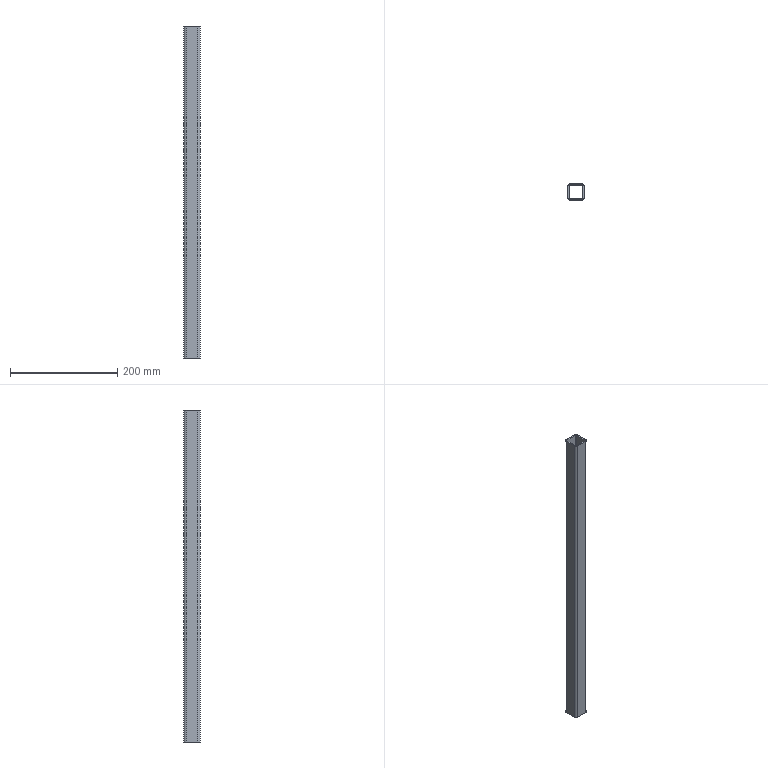Part | NX | features DATUM_CSYS 2, EXTRUDE 1, MOVE_FACE 1, SKETCH 1 | 1 solid | 18 faces | box 30 x 30 x 620 mm | volume 132493 mm3 | plane 10 | cylinder 8 | commonest cylinder face diameters 4 x4 8 x4
STEP:
#1=CARTESIAN_POINT('',(15.,11.,620.));
#2=VERTEX_POINT('',#1);
#3=CARTESIAN_POINT('',(11.,15.,620.));
#4=VERTEX_POINT('',#3);
#5=CARTESIAN_POINT('',(11.,11.,620.));
#6=DIRECTION('',(0.,0.,1.));
#7=DIRECTION('',(1.,0.,0.));
#8=AXIS2_PLACEMENT_3D('',#5,#6,#7);
#9=CIRCLE('',#8,4.);
#10=EDGE_CURVE('',#2,#4,#9,.T.);
#11=ORIENTED_EDGE('',*,*,#10,.T.);
#12=CARTESIAN_POINT('',(-11.,15.,620.));
#13=VERTEX_POINT('',#12);
#14=CARTESIAN_POINT('',(11.,15.,620.));
#15=DIRECTION('',(-1.,0.,0.));
#16=VECTOR('',#15,1000.);
#17=LINE('',#14,#16);
#18=EDGE_CURVE('',#4,#13,#17,.T.);
#19=ORIENTED_EDGE('',*,*,#18,.T.);
#20=CARTESIAN_POINT('',(-15.,11.,620.));
#21=VERTEX_POINT('',#20);
#22=CARTESIAN_POINT('',(-11.,11.,620.));
#23=DIRECTION('',(0.,0.,1.));
#24=DIRECTION('',(1.,0.,0.));
#25=AXIS2_PLACEMENT_3D('',#22,#23,#24);
#26=CIRCLE('',#25,4.);
#27=EDGE_CURVE('',#13,#21,#26,.T.);
#28=ORIENTED_EDGE('',*,*,#27,.T.);
#29=CARTESIAN_POINT('',(-15.,-11.,620.));
#30=VERTEX_POINT('',#29);
#31=CARTESIAN_POINT('',(-15.,11.,620.));
#32=DIRECTION('',(0.,-1.,0.));
#33=VECTOR('',#32,1000.);
#34=LINE('',#31,#33);
#35=EDGE_CURVE('',#21,#30,#34,.T.);
#36=ORIENTED_EDGE('',*,*,#35,.T.);
#37=CARTESIAN_POINT('',(-11.,-15.,620.));
#38=VERTEX_POINT('',#37);
#39=CARTESIAN_POINT('',(-11.,-11.,620.));
#40=DIRECTION('',(0.,0.,1.));
#41=DIRECTION('',(1.,0.,0.));
#42=AXIS2_PLACEMENT_3D('',#39,#40,#41);
#43=CIRCLE('',#42,4.);
#44=EDGE_CURVE('',#30,#38,#43,.T.);
#45=ORIENTED_EDGE('',*,*,#44,.T.);
#46=CARTESIAN_POINT('',(11.,-15.,620.));
#47=VERTEX_POINT('',#46);
#48=CARTESIAN_POINT('',(-11.,-15.,620.));
#49=DIRECTION('',(1.,0.,0.));
#50=VECTOR('',#49,1000.);
#51=LINE('',#48,#50);
#52=EDGE_CURVE('',#38,#47,#51,.T.);
#53=ORIENTED_EDGE('',*,*,#52,.T.);
#54=CARTESIAN_POINT('',(15.,-11.,620.));
#55=VERTEX_POINT('',#54);
#56=CARTESIAN_POINT('',(11.,-11.,620.));
#57=DIRECTION('',(0.,0.,1.));
#58=DIRECTION('',(1.,0.,0.));
#59=AXIS2_PLACEMENT_3D('',#56,#57,#58);
#60=CIRCLE('',#59,4.);
#61=EDGE_CURVE('',#47,#55,#60,.T.);
#62=ORIENTED_EDGE('',*,*,#61,.T.);
#63=CARTESIAN_POINT('',(15.,-11.,620.));
#64=DIRECTION('',(0.,1.,0.));
#65=VECTOR('',#64,1000.);
#66=LINE('',#63,#65);
#67=EDGE_CURVE('',#55,#2,#66,.T.);
#68=ORIENTED_EDGE('',*,*,#67,.T.);
#69=EDGE_LOOP('',(#11,#19,#28,#36,#45,#53,#62,#68));
#70=FACE_BOUND('',#69,.T.);
#71=CARTESIAN_POINT('',(13.,11.,620.));
#72=VERTEX_POINT('',#71);
#73=CARTESIAN_POINT('',(11.,13.,620.));
#74=VERTEX_POINT('',#73);
#75=CARTESIAN_POINT('',(11.,11.,620.));
#76=DIRECTION('',(0.,0.,1.));
#77=DIRECTION('',(1.,0.,0.));
#78=AXIS2_PLACEMENT_3D('',#75,#76,#77);
#79=CIRCLE('',#78,2.);
#80=EDGE_CURVE('',#72,#74,#79,.T.);
#81=ORIENTED_EDGE('',*,*,#80,.F.);
#82=CARTESIAN_POINT('',(13.,-11.,620.));
#83=VERTEX_POINT('',#82);
#84=CARTESIAN_POINT('',(13.,-11.,620.));
#85=DIRECTION('',(0.,1.,0.));
#86=VECTOR('',#85,1000.);
#87=LINE('',#84,#86);
#88=EDGE_CURVE('',#83,#72,#87,.T.);
#89=ORIENTED_EDGE('',*,*,#88,.F.);
#90=CARTESIAN_POINT('',(11.,-13.,620.));
#91=VERTEX_POINT('',#90);
#92=CARTESIAN_POINT('',(11.,-11.,620.));
#93=DIRECTION('',(0.,0.,1.));
#94=DIRECTION('',(1.,0.,0.));
#95=AXIS2_PLACEMENT_3D('',#92,#93,#94);
#96=CIRCLE('',#95,2.);
#97=EDGE_CURVE('',#91,#83,#96,.T.);
#98=ORIENTED_EDGE('',*,*,#97,.F.);
#99=CARTESIAN_POINT('',(-11.,-13.,620.));
#100=VERTEX_POINT('',#99);
#101=CARTESIAN_POINT('',(-11.,-13.,620.));
#102=DIRECTION('',(1.,0.,0.));
#103=VECTOR('',#102,1000.);
#104=LINE('',#101,#103);
#105=EDGE_CURVE('',#100,#91,#104,.T.);
#106=ORIENTED_EDGE('',*,*,#105,.F.);
#107=CARTESIAN_POINT('',(-13.,-11.,620.));
#108=VERTEX_POINT('',#107);
#109=CARTESIAN_POINT('',(-11.,-11.,620.));
#110=DIRECTION('',(0.,0.,1.));
#111=DIRECTION('',(1.,0.,0.));
#112=AXIS2_PLACEMENT_3D('',#109,#110,#111);
#113=CIRCLE('',#112,2.);
#114=EDGE_CURVE('',#108,#100,#113,.T.);
#115=ORIENTED_EDGE('',*,*,#114,.F.);
#116=CARTESIAN_POINT('',(-13.,11.,620.));
#117=VERTEX_POINT('',#116);
#118=CARTESIAN_POINT('',(-13.,11.,620.));
#119=DIRECTION('',(0.,-1.,0.));
#120=VECTOR('',#119,1000.);
#121=LINE('',#118,#120);
#122=EDGE_CURVE('',#117,#108,#121,.T.);
#123=ORIENTED_EDGE('',*,*,#122,.F.);
#124=CARTESIAN_POINT('',(-11.,13.,620.));
#125=VERTEX_POINT('',#124);
#126=CARTESIAN_POINT('',(-11.,11.,620.));
#127=DIRECTION('',(0.,0.,1.));
#128=DIRECTION('',(1.,0.,0.));
#129=AXIS2_PLACEMENT_3D('',#126,#127,#128);
#130=CIRCLE('',#129,2.);
#131=EDGE_CURVE('',#125,#117,#130,.T.);
#132=ORIENTED_EDGE('',*,*,#131,.F.);
#133=CARTESIAN_POINT('',(11.,13.,620.));
#134=DIRECTION('',(-1.,0.,0.));
#135=VECTOR('',#134,1000.);
#136=LINE('',#133,#135);
#137=EDGE_CURVE('',#74,#125,#136,.T.);
#138=ORIENTED_EDGE('',*,*,#137,.F.);
#139=EDGE_LOOP('',(#81,#89,#98,#106,#115,#123,#132,#138));
#140=FACE_BOUND('',#139,.T.);
#141=CARTESIAN_POINT('',(11.,11.,620.));
#142=DIRECTION('',(0.,0.,-1.));
#143=DIRECTION('',(-1.,0.,0.));
#144=AXIS2_PLACEMENT_3D('',#141,#142,#143);
#145=PLANE('',#144);
#146=ADVANCED_FACE('',(#70,#140),#145,.F.);
#147=CARTESIAN_POINT('',(-11.,15.,0.));
#148=VERTEX_POINT('',#147);
#149=CARTESIAN_POINT('',(-15.,11.,0.));
#150=VERTEX_POINT('',#149);
#151=CARTESIAN_POINT('',(-11.,11.,0.));
#152=DIRECTION('',(0.,0.,1.));
#153=DIRECTION('',(1.,0.,0.));
#154=AXIS2_PLACEMENT_3D('',#151,#152,#153);
#155=CIRCLE('',#154,4.);
#156=EDGE_CURVE('',#148,#150,#155,.T.);
#157=ORIENTED_EDGE('',*,*,#156,.F.);
#158=CARTESIAN_POINT('',(11.,15.,0.));
#159=VERTEX_POINT('',#158);
#160=CARTESIAN_POINT('',(11.,15.,0.));
#161=DIRECTION('',(-1.,0.,0.));
#162=VECTOR('',#161,1000.);
#163=LINE('',#160,#162);
#164=EDGE_CURVE('',#159,#148,#163,.T.);
#165=ORIENTED_EDGE('',*,*,#164,.F.);
#166=CARTESIAN_POINT('',(15.,11.,0.));
#167=VERTEX_POINT('',#166);
#168=CARTESIAN_POINT('',(11.,11.,0.));
#169=DIRECTION('',(0.,0.,1.));
#170=DIRECTION('',(1.,0.,0.));
#171=AXIS2_PLACEMENT_3D('',#168,#169,#170);
#172=CIRCLE('',#171,4.);
#173=EDGE_CURVE('',#167,#159,#172,.T.);
#174=ORIENTED_EDGE('',*,*,#173,.F.);
#175=CARTESIAN_POINT('',(15.,-11.,0.));
#176=VERTEX_POINT('',#175);
#177=CARTESIAN_POINT('',(15.,-11.,0.));
#178=DIRECTION('',(0.,1.,0.));
#179=VECTOR('',#178,1000.);
#180=LINE('',#177,#179);
#181=EDGE_CURVE('',#176,#167,#180,.T.);
#182=ORIENTED_EDGE('',*,*,#181,.F.);
#183=CARTESIAN_POINT('',(11.,-15.,0.));
#184=VERTEX_POINT('',#183);
#185=CARTESIAN_POINT('',(11.,-11.,0.));
#186=DIRECTION('',(0.,0.,1.));
#187=DIRECTION('',(1.,0.,0.));
#188=AXIS2_PLACEMENT_3D('',#185,#186,#187);
#189=CIRCLE('',#188,4.);
#190=EDGE_CURVE('',#184,#176,#189,.T.);
#191=ORIENTED_EDGE('',*,*,#190,.F.);
#192=CARTESIAN_POINT('',(-11.,-15.,0.));
#193=VERTEX_POINT('',#192);
#194=CARTESIAN_POINT('',(-11.,-15.,0.));
#195=DIRECTION('',(1.,0.,0.));
#196=VECTOR('',#195,1000.);
#197=LINE('',#194,#196);
#198=EDGE_CURVE('',#193,#184,#197,.T.);
#199=ORIENTED_EDGE('',*,*,#198,.F.);
#200=CARTESIAN_POINT('',(-15.,-11.,0.));
#201=VERTEX_POINT('',#200);
#202=CARTESIAN_POINT('',(-11.,-11.,0.));
#203=DIRECTION('',(0.,0.,1.));
#204=DIRECTION('',(1.,0.,0.));
#205=AXIS2_PLACEMENT_3D('',#202,#203,#204);
#206=CIRCLE('',#205,4.);
#207=EDGE_CURVE('',#201,#193,#206,.T.);
#208=ORIENTED_EDGE('',*,*,#207,.F.);
#209=CARTESIAN_POINT('',(-15.,11.,0.));
#210=DIRECTION('',(0.,-1.,0.));
#211=VECTOR('',#210,1000.);
#212=LINE('',#209,#211);
#213=EDGE_CURVE('',#150,#201,#212,.T.);
#214=ORIENTED_EDGE('',*,*,#213,.F.);
#215=EDGE_LOOP('',(#157,#165,#174,#182,#191,#199,#208,#214));
#216=FACE_BOUND('',#215,.T.);
#217=CARTESIAN_POINT('',(-11.,13.,0.));
#218=VERTEX_POINT('',#217);
#219=CARTESIAN_POINT('',(-13.,11.,0.));
#220=VERTEX_POINT('',#219);
#221=CARTESIAN_POINT('',(-11.,11.,0.));
#222=DIRECTION('',(0.,0.,1.));
#223=DIRECTION('',(1.,0.,0.));
#224=AXIS2_PLACEMENT_3D('',#221,#222,#223);
#225=CIRCLE('',#224,2.);
#226=EDGE_CURVE('',#218,#220,#225,.T.);
#227=ORIENTED_EDGE('',*,*,#226,.T.);
#228=CARTESIAN_POINT('',(-13.,-11.,0.));
#229=VERTEX_POINT('',#228);
#230=CARTESIAN_POINT('',(-13.,11.,0.));
#231=DIRECTION('',(0.,-1.,0.));
#232=VECTOR('',#231,1000.);
#233=LINE('',#230,#232);
#234=EDGE_CURVE('',#220,#229,#233,.T.);
#235=ORIENTED_EDGE('',*,*,#234,.T.);
#236=CARTESIAN_POINT('',(-11.,-13.,0.));
#237=VERTEX_POINT('',#236);
#238=CARTESIAN_POINT('',(-11.,-11.,0.));
#239=DIRECTION('',(0.,0.,1.));
#240=DIRECTION('',(1.,0.,0.));
#241=AXIS2_PLACEMENT_3D('',#238,#239,#240);
#242=CIRCLE('',#241,2.);
#243=EDGE_CURVE('',#229,#237,#242,.T.);
#244=ORIENTED_EDGE('',*,*,#243,.T.);
#245=CARTESIAN_POINT('',(11.,-13.,0.));
#246=VERTEX_POINT('',#245);
#247=CARTESIAN_POINT('',(-11.,-13.,0.));
#248=DIRECTION('',(1.,0.,0.));
#249=VECTOR('',#248,1000.);
#250=LINE('',#247,#249);
#251=EDGE_CURVE('',#237,#246,#250,.T.);
#252=ORIENTED_EDGE('',*,*,#251,.T.);
#253=CARTESIAN_POINT('',(13.,-11.,0.));
#254=VERTEX_POINT('',#253);
#255=CARTESIAN_POINT('',(11.,-11.,0.));
#256=DIRECTION('',(0.,0.,1.));
#257=DIRECTION('',(1.,0.,0.));
#258=AXIS2_PLACEMENT_3D('',#255,#256,#257);
#259=CIRCLE('',#258,2.);
#260=EDGE_CURVE('',#246,#254,#259,.T.);
#261=ORIENTED_EDGE('',*,*,#260,.T.);
#262=CARTESIAN_POINT('',(13.,11.,0.));
#263=VERTEX_POINT('',#262);
#264=CARTESIAN_POINT('',(13.,-11.,0.));
#265=DIRECTION('',(0.,1.,0.));
#266=VECTOR('',#265,1000.);
#267=LINE('',#264,#266);
#268=EDGE_CURVE('',#254,#263,#267,.T.);
#269=ORIENTED_EDGE('',*,*,#268,.T.);
#270=CARTESIAN_POINT('',(11.,13.,0.));
#271=VERTEX_POINT('',#270);
#272=CARTESIAN_POINT('',(11.,11.,0.));
#273=DIRECTION('',(0.,0.,1.));
#274=DIRECTION('',(1.,0.,0.));
#275=AXIS2_PLACEMENT_3D('',#272,#273,#274);
#276=CIRCLE('',#275,2.);
#277=EDGE_CURVE('',#263,#271,#276,.T.);
#278=ORIENTED_EDGE('',*,*,#277,.T.);
#279=CARTESIAN_POINT('',(11.,13.,0.));
#280=DIRECTION('',(-1.,0.,0.));
#281=VECTOR('',#280,1000.);
#282=LINE('',#279,#281);
#283=EDGE_CURVE('',#271,#218,#282,.T.);
#284=ORIENTED_EDGE('',*,*,#283,.T.);
#285=EDGE_LOOP('',(#227,#235,#244,#252,#261,#269,#278,#284));
#286=FACE_BOUND('',#285,.T.);
#287=CARTESIAN_POINT('',(-11.,11.,0.));
#288=DIRECTION('',(0.,0.,-1.));
#289=DIRECTION('',(-1.,0.,0.));
#290=AXIS2_PLACEMENT_3D('',#287,#288,#289);
#291=PLANE('',#290);
#292=ADVANCED_FACE('',(#216,#286),#291,.T.);
#293=ORIENTED_EDGE('',*,*,#18,.F.);
#294=CARTESIAN_POINT('',(11.,15.,0.));
#295=DIRECTION('',(0.,0.,1.));
#296=VECTOR('',#295,1000.);
#297=LINE('',#294,#296);
#298=EDGE_CURVE('',#159,#4,#297,.T.);
#299=ORIENTED_EDGE('',*,*,#298,.F.);
#300=ORIENTED_EDGE('',*,*,#164,.T.);
#301=CARTESIAN_POINT('',(-11.,15.,0.));
#302=DIRECTION('',(0.,0.,1.));
#303=VECTOR('',#302,1000.);
#304=LINE('',#301,#303);
#305=EDGE_CURVE('',#148,#13,#304,.T.);
#306=ORIENTED_EDGE('',*,*,#305,.T.);
#307=EDGE_LOOP('',(#293,#299,#300,#306));
#308=FACE_BOUND('',#307,.T.);
#309=CARTESIAN_POINT('',(11.,15.,0.));
#310=DIRECTION('',(0.,1.,0.));
#311=DIRECTION('',(-1.,0.,0.));
#312=AXIS2_PLACEMENT_3D('',#309,#310,#311);
#313=PLANE('',#312);
#314=ADVANCED_FACE('',(#308),#313,.T.);
#315=ORIENTED_EDGE('',*,*,#27,.F.);
#316=ORIENTED_EDGE('',*,*,#305,.F.);
#317=ORIENTED_EDGE('',*,*,#156,.T.);
#318=CARTESIAN_POINT('',(-15.,11.,0.));
#319=DIRECTION('',(0.,0.,1.));
#320=VECTOR('',#319,1000.);
#321=LINE('',#318,#320);
#322=EDGE_CURVE('',#150,#21,#321,.T.);
#323=ORIENTED_EDGE('',*,*,#322,.T.);
#324=EDGE_LOOP('',(#315,#316,#317,#323));
#325=FACE_BOUND('',#324,.T.);
#326=CARTESIAN_POINT('',(-11.,11.,0.));
#327=DIRECTION('',(0.,0.,1.));
#328=DIRECTION('',(1.,0.,0.));
#329=AXIS2_PLACEMENT_3D('',#326,#327,#328);
#330=CYLINDRICAL_SURFACE('',#329,4.);
#331=ADVANCED_FACE('',(#325),#330,.T.);
#332=ORIENTED_EDGE('',*,*,#35,.F.);
#333=ORIENTED_EDGE('',*,*,#322,.F.);
#334=ORIENTED_EDGE('',*,*,#213,.T.);
#335=CARTESIAN_POINT('',(-15.,-11.,0.));
#336=DIRECTION('',(0.,0.,1.));
#337=VECTOR('',#336,1000.);
#338=LINE('',#335,#337);
#339=EDGE_CURVE('',#201,#30,#338,.T.);
#340=ORIENTED_EDGE('',*,*,#339,.T.);
#341=EDGE_LOOP('',(#332,#333,#334,#340));
#342=FACE_BOUND('',#341,.T.);
#343=CARTESIAN_POINT('',(-15.,11.,0.));
#344=DIRECTION('',(-1.,0.,0.));
#345=DIRECTION('',(0.,-1.,0.));
#346=AXIS2_PLACEMENT_3D('',#343,#344,#345);
#347=PLANE('',#346);
#348=ADVANCED_FACE('',(#342),#347,.T.);
#349=ORIENTED_EDGE('',*,*,#44,.F.);
#350=ORIENTED_EDGE('',*,*,#339,.F.);
#351=ORIENTED_EDGE('',*,*,#207,.T.);
#352=CARTESIAN_POINT('',(-11.,-15.,0.));
#353=DIRECTION('',(0.,0.,1.));
#354=VECTOR('',#353,1000.);
#355=LINE('',#352,#354);
#356=EDGE_CURVE('',#193,#38,#355,.T.);
#357=ORIENTED_EDGE('',*,*,#356,.T.);
#358=EDGE_LOOP('',(#349,#350,#351,#357));
#359=FACE_BOUND('',#358,.T.);
#360=CARTESIAN_POINT('',(-11.,-11.,0.));
#361=DIRECTION('',(0.,0.,1.));
#362=DIRECTION('',(1.,0.,0.));
#363=AXIS2_PLACEMENT_3D('',#360,#361,#362);
#364=CYLINDRICAL_SURFACE('',#363,4.);
#365=ADVANCED_FACE('',(#359),#364,.T.);
#366=ORIENTED_EDGE('',*,*,#52,.F.);
#367=ORIENTED_EDGE('',*,*,#356,.F.);
#368=ORIENTED_EDGE('',*,*,#198,.T.);
#369=CARTESIAN_POINT('',(11.,-15.,0.));
#370=DIRECTION('',(0.,0.,1.));
#371=VECTOR('',#370,1000.);
#372=LINE('',#369,#371);
#373=EDGE_CURVE('',#184,#47,#372,.T.);
#374=ORIENTED_EDGE('',*,*,#373,.T.);
#375=EDGE_LOOP('',(#366,#367,#368,#374));
#376=FACE_BOUND('',#375,.T.);
#377=CARTESIAN_POINT('',(-11.,-15.,0.));
#378=DIRECTION('',(0.,-1.,0.));
#379=DIRECTION('',(1.,0.,0.));
#380=AXIS2_PLACEMENT_3D('',#377,#378,#379);
#381=PLANE('',#380);
#382=ADVANCED_FACE('',(#376),#381,.T.);
#383=ORIENTED_EDGE('',*,*,#61,.F.);
#384=ORIENTED_EDGE('',*,*,#373,.F.);
#385=ORIENTED_EDGE('',*,*,#190,.T.);
#386=CARTESIAN_POINT('',(15.,-11.,0.));
#387=DIRECTION('',(0.,0.,1.));
#388=VECTOR('',#387,1000.);
#389=LINE('',#386,#388);
#390=EDGE_CURVE('',#176,#55,#389,.T.);
#391=ORIENTED_EDGE('',*,*,#390,.T.);
#392=EDGE_LOOP('',(#383,#384,#385,#391));
#393=FACE_BOUND('',#392,.T.);
#394=CARTESIAN_POINT('',(11.,-11.,0.));
#395=DIRECTION('',(0.,0.,1.));
#396=DIRECTION('',(1.,0.,0.));
#397=AXIS2_PLACEMENT_3D('',#394,#395,#396);
#398=CYLINDRICAL_SURFACE('',#397,4.);
#399=ADVANCED_FACE('',(#393),#398,.T.);
#400=ORIENTED_EDGE('',*,*,#67,.F.);
#401=ORIENTED_EDGE('',*,*,#390,.F.);
#402=ORIENTED_EDGE('',*,*,#181,.T.);
#403=CARTESIAN_POINT('',(15.,11.,0.));
#404=DIRECTION('',(0.,0.,1.));
#405=VECTOR('',#404,1000.);
#406=LINE('',#403,#405);
#407=EDGE_CURVE('',#167,#2,#406,.T.);
#408=ORIENTED_EDGE('',*,*,#407,.T.);
#409=EDGE_LOOP('',(#400,#401,#402,#408));
#410=FACE_BOUND('',#409,.T.);
#411=CARTESIAN_POINT('',(15.,-11.,0.));
#412=DIRECTION('',(1.,0.,0.));
#413=DIRECTION('',(0.,0.,-1.));
#414=AXIS2_PLACEMENT_3D('',#411,#412,#413);
#415=PLANE('',#414);
#416=ADVANCED_FACE('',(#410),#415,.T.);
#417=ORIENTED_EDGE('',*,*,#10,.F.);
#418=ORIENTED_EDGE('',*,*,#407,.F.);
#419=ORIENTED_EDGE('',*,*,#173,.T.);
#420=ORIENTED_EDGE('',*,*,#298,.T.);
#421=EDGE_LOOP('',(#417,#418,#419,#420));
#422=FACE_BOUND('',#421,.T.);
#423=CARTESIAN_POINT('',(11.,11.,0.));
#424=DIRECTION('',(0.,0.,1.));
#425=DIRECTION('',(1.,0.,0.));
#426=AXIS2_PLACEMENT_3D('',#423,#424,#425);
#427=CYLINDRICAL_SURFACE('',#426,4.);
#428=ADVANCED_FACE('',(#422),#427,.T.);
#429=ORIENTED_EDGE('',*,*,#137,.T.);
#430=CARTESIAN_POINT('',(-11.,13.,0.));
#431=DIRECTION('',(0.,0.,1.));
#432=VECTOR('',#431,1000.);
#433=LINE('',#430,#432);
#434=EDGE_CURVE('',#218,#125,#433,.T.);
#435=ORIENTED_EDGE('',*,*,#434,.F.);
#436=ORIENTED_EDGE('',*,*,#283,.F.);
#437=CARTESIAN_POINT('',(11.,13.,0.));
#438=DIRECTION('',(0.,0.,1.));
#439=VECTOR('',#438,1000.);
#440=LINE('',#437,#439);
#441=EDGE_CURVE('',#271,#74,#440,.T.);
#442=ORIENTED_EDGE('',*,*,#441,.T.);
#443=EDGE_LOOP('',(#429,#435,#436,#442));
#444=FACE_BOUND('',#443,.T.);
#445=CARTESIAN_POINT('',(11.,13.,0.));
#446=DIRECTION('',(0.,1.,0.));
#447=DIRECTION('',(-1.,0.,0.));
#448=AXIS2_PLACEMENT_3D('',#445,#446,#447);
#449=PLANE('',#448);
#450=ADVANCED_FACE('',(#444),#449,.F.);
#451=ORIENTED_EDGE('',*,*,#131,.T.);
#452=CARTESIAN_POINT('',(-13.,11.,0.));
#453=DIRECTION('',(0.,0.,1.));
#454=VECTOR('',#453,1000.);
#455=LINE('',#452,#454);
#456=EDGE_CURVE('',#220,#117,#455,.T.);
#457=ORIENTED_EDGE('',*,*,#456,.F.);
#458=ORIENTED_EDGE('',*,*,#226,.F.);
#459=ORIENTED_EDGE('',*,*,#434,.T.);
#460=EDGE_LOOP('',(#451,#457,#458,#459));
#461=FACE_BOUND('',#460,.T.);
#462=CARTESIAN_POINT('',(-11.,11.,0.));
#463=DIRECTION('',(0.,0.,1.));
#464=DIRECTION('',(1.,0.,0.));
#465=AXIS2_PLACEMENT_3D('',#462,#463,#464);
#466=CYLINDRICAL_SURFACE('',#465,2.);
#467=ADVANCED_FACE('',(#461),#466,.F.);
#468=ORIENTED_EDGE('',*,*,#122,.T.);
#469=CARTESIAN_POINT('',(-13.,-11.,0.));
#470=DIRECTION('',(0.,0.,1.));
#471=VECTOR('',#470,1000.);
#472=LINE('',#469,#471);
#473=EDGE_CURVE('',#229,#108,#472,.T.);
#474=ORIENTED_EDGE('',*,*,#473,.F.);
#475=ORIENTED_EDGE('',*,*,#234,.F.);
#476=ORIENTED_EDGE('',*,*,#456,.T.);
#477=EDGE_LOOP('',(#468,#474,#475,#476));
#478=FACE_BOUND('',#477,.T.);
#479=CARTESIAN_POINT('',(-13.,11.,0.));
#480=DIRECTION('',(-1.,0.,0.));
#481=DIRECTION('',(0.,-1.,0.));
#482=AXIS2_PLACEMENT_3D('',#479,#480,#481);
#483=PLANE('',#482);
#484=ADVANCED_FACE('',(#478),#483,.F.);
#485=ORIENTED_EDGE('',*,*,#114,.T.);
#486=CARTESIAN_POINT('',(-11.,-13.,0.));
#487=DIRECTION('',(0.,0.,1.));
#488=VECTOR('',#487,1000.);
#489=LINE('',#486,#488);
#490=EDGE_CURVE('',#237,#100,#489,.T.);
#491=ORIENTED_EDGE('',*,*,#490,.F.);
#492=ORIENTED_EDGE('',*,*,#243,.F.);
#493=ORIENTED_EDGE('',*,*,#473,.T.);
#494=EDGE_LOOP('',(#485,#491,#492,#493));
#495=FACE_BOUND('',#494,.T.);
#496=CARTESIAN_POINT('',(-11.,-11.,0.));
#497=DIRECTION('',(0.,0.,1.));
#498=DIRECTION('',(1.,0.,0.));
#499=AXIS2_PLACEMENT_3D('',#496,#497,#498);
#500=CYLINDRICAL_SURFACE('',#499,2.);
#501=ADVANCED_FACE('',(#495),#500,.F.);
#502=ORIENTED_EDGE('',*,*,#105,.T.);
#503=CARTESIAN_POINT('',(11.,-13.,0.));
#504=DIRECTION('',(0.,0.,1.));
#505=VECTOR('',#504,1000.);
#506=LINE('',#503,#505);
#507=EDGE_CURVE('',#246,#91,#506,.T.);
#508=ORIENTED_EDGE('',*,*,#507,.F.);
#509=ORIENTED_EDGE('',*,*,#251,.F.);
#510=ORIENTED_EDGE('',*,*,#490,.T.);
#511=EDGE_LOOP('',(#502,#508,#509,#510));
#512=FACE_BOUND('',#511,.T.);
#513=CARTESIAN_POINT('',(-11.,-13.,0.));
#514=DIRECTION('',(0.,-1.,0.));
#515=DIRECTION('',(1.,0.,0.));
#516=AXIS2_PLACEMENT_3D('',#513,#514,#515);
#517=PLANE('',#516);
#518=ADVANCED_FACE('',(#512),#517,.F.);
#519=ORIENTED_EDGE('',*,*,#97,.T.);
#520=CARTESIAN_POINT('',(13.,-11.,0.));
#521=DIRECTION('',(0.,0.,1.));
#522=VECTOR('',#521,1000.);
#523=LINE('',#520,#522);
#524=EDGE_CURVE('',#254,#83,#523,.T.);
#525=ORIENTED_EDGE('',*,*,#524,.F.);
#526=ORIENTED_EDGE('',*,*,#260,.F.);
#527=ORIENTED_EDGE('',*,*,#507,.T.);
#528=EDGE_LOOP('',(#519,#525,#526,#527));
#529=FACE_BOUND('',#528,.T.);
#530=CARTESIAN_POINT('',(11.,-11.,0.));
#531=DIRECTION('',(0.,0.,1.));
#532=DIRECTION('',(1.,0.,0.));
#533=AXIS2_PLACEMENT_3D('',#530,#531,#532);
#534=CYLINDRICAL_SURFACE('',#533,2.);
#535=ADVANCED_FACE('',(#529),#534,.F.);
#536=ORIENTED_EDGE('',*,*,#88,.T.);
#537=CARTESIAN_POINT('',(13.,11.,0.));
#538=DIRECTION('',(0.,0.,-1.));
#539=VECTOR('',#538,1000.);
#540=LINE('',#537,#539);
#541=EDGE_CURVE('',#263,#72,#540,.F.);
#542=ORIENTED_EDGE('',*,*,#541,.F.);
#543=ORIENTED_EDGE('',*,*,#268,.F.);
#544=ORIENTED_EDGE('',*,*,#524,.T.);
#545=EDGE_LOOP('',(#536,#542,#543,#544));
#546=FACE_BOUND('',#545,.T.);
#547=CARTESIAN_POINT('',(13.,-11.,0.));
#548=DIRECTION('',(1.,0.,0.));
#549=DIRECTION('',(0.,0.,-1.));
#550=AXIS2_PLACEMENT_3D('',#547,#548,#549);
#551=PLANE('',#550);
#552=ADVANCED_FACE('',(#546),#551,.F.);
#553=ORIENTED_EDGE('',*,*,#80,.T.);
#554=ORIENTED_EDGE('',*,*,#441,.F.);
#555=ORIENTED_EDGE('',*,*,#277,.F.);
#556=ORIENTED_EDGE('',*,*,#541,.T.);
#557=EDGE_LOOP('',(#553,#554,#555,#556));
#558=FACE_BOUND('',#557,.T.);
#559=CARTESIAN_POINT('',(11.,11.,0.));
#560=DIRECTION('',(0.,0.,1.));
#561=DIRECTION('',(1.,0.,0.));
#562=AXIS2_PLACEMENT_3D('',#559,#560,#561);
#563=CYLINDRICAL_SURFACE('',#562,2.);
#564=ADVANCED_FACE('',(#558),#563,.F.);
#565=CLOSED_SHELL('',(#146,#292,#314,#331,#348,#365,#382,#399,#416,#428,#450,#467,#484,#501,#518,#535,#552,#564));
#566=MANIFOLD_SOLID_BREP('',#565);
#567=(LENGTH_UNIT()NAMED_UNIT(*)SI_UNIT(.MILLI.,.METRE.));
#568=UNCERTAINTY_MEASURE_WITH_UNIT(LENGTH_MEASURE(0.00001),#567,'','');
#569=(NAMED_UNIT(*)PLANE_ANGLE_UNIT()SI_UNIT($,.RADIAN.));
#570=(NAMED_UNIT(*)SI_UNIT($,.STERADIAN.)SOLID_ANGLE_UNIT());
#571=(GEOMETRIC_REPRESENTATION_CONTEXT(3)GLOBAL_UNCERTAINTY_ASSIGNED_CONTEXT((#568))GLOBAL_UNIT_ASSIGNED_CONTEXT((#567,#569,#570))REPRESENTATION_CONTEXT('',''));
#572=ADVANCED_BREP_SHAPE_REPRESENTATION('',(#566),#571);